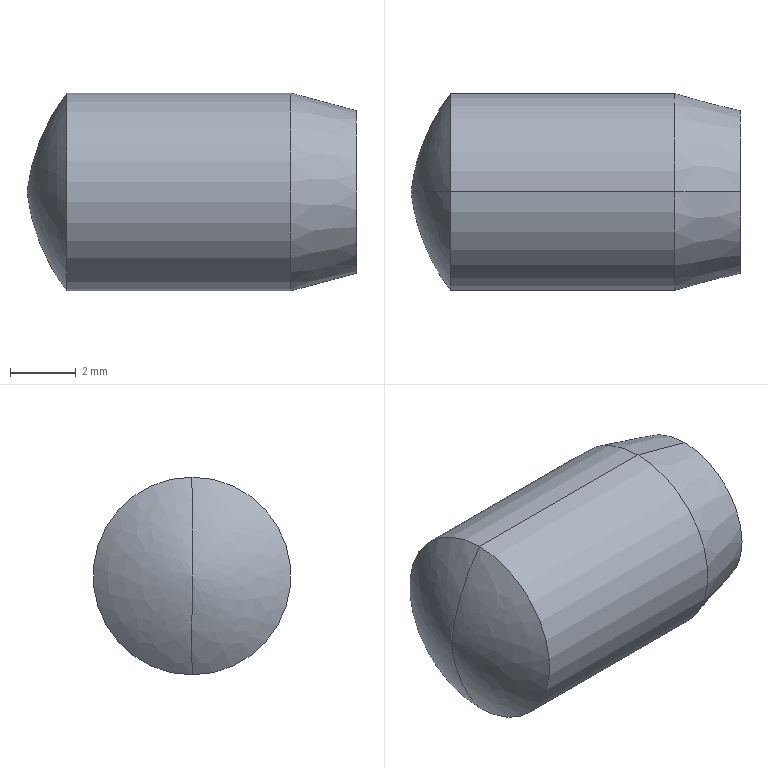Part | STEP file | 0245_020_MSC6-10 | 1 solid | 7 faces | box 10 x 6 x 6 mm | volume 255.239 mm3 | spline 2 | cylinder 2 | cone 2 | plane 1 | commonest cylinder face diameters 6 x2
STEP:
#1=CARTESIAN_POINT('',(0.,0.,0.));
#2=DIRECTION('',(0.,0.,1.));
#3=DIRECTION('',(1.,0.,0.));
#4=AXIS2_PLACEMENT_3D('',#1,#2,#3);
#5=CARTESIAN_POINT('',(-5.,0.,0.));
#6=VERTEX_POINT('',#5);
#7=CARTESIAN_POINT('',(-3.8,0.,3.));
#8=VERTEX_POINT('',#7);
#9=CARTESIAN_POINT('',(0.9651,0.,-0.646));
#10=DIRECTION('',(0.,1.,0.));
#11=DIRECTION('',(0.,0.,1.));
#12=AXIS2_PLACEMENT_3D('',#9,#10,#11);
#13=CIRCLE('',#12,6.);
#14=CARTESIAN_POINT('',(-5.,0.,0.));
#15=CARTESIAN_POINT('',(-5.,0.,0.));
#16=CARTESIAN_POINT('',(-5.,0.,0.));
#17=CARTESIAN_POINT('',(-5.,0.,0.));
#18=CARTESIAN_POINT('',(-4.881,0.,-1.098));
#19=CARTESIAN_POINT('',(-4.881,-2.196,-1.098));
#20=CARTESIAN_POINT('',(-4.881,-2.196,1.098));
#21=CARTESIAN_POINT('',(-4.881,0.,1.098));
#22=CARTESIAN_POINT('',(-4.471,0.,-2.123));
#23=CARTESIAN_POINT('',(-4.471,-4.246,-2.123));
#24=CARTESIAN_POINT('',(-4.471,-4.246,2.123));
#25=CARTESIAN_POINT('',(-4.471,0.,2.123));
#26=CARTESIAN_POINT('',(-3.8,0.,-3.));
#27=CARTESIAN_POINT('',(-3.8,-6.,-3.));
#28=CARTESIAN_POINT('',(-3.8,-6.,3.));
#29=CARTESIAN_POINT('',(-3.8,0.,3.));
#30=(BOUNDED_SURFACE()B_SPLINE_SURFACE(3,3,((#14,#15,#16,#17),(#18,#19,#20,#21),(#22,#23,#24,#25),(#26,#27,#28,#29)),.UNSPECIFIED.,.F.,.F.,.F.)B_SPLINE_SURFACE_WITH_KNOTS((4,4),(4,4),(0.,1.),(0.,1.),.PIECEWISE_BEZIER_KNOTS.)GEOMETRIC_REPRESENTATION_ITEM()RATIONAL_B_SPLINE_SURFACE(((1.,0.3333,0.3333,1.),(0.9754,0.3251,0.3251,0.9754),(0.9754,0.3251,0.3251,0.9754),(1.,0.3333,0.3333,1.)))REPRESENTATION_ITEM('')SURFACE());
#31=CARTESIAN_POINT('',(0.,1.));
#32=CARTESIAN_POINT('',(0.01534,1.));
#33=CARTESIAN_POINT('',(0.04597,1.));
#34=CARTESIAN_POINT('',(0.09177,1.));
#35=CARTESIAN_POINT('',(0.1374,1.));
#36=CARTESIAN_POINT('',(0.183,1.));
#37=CARTESIAN_POINT('',(0.2285,1.));
#38=CARTESIAN_POINT('',(0.2739,1.));
#39=CARTESIAN_POINT('',(0.3192,1.));
#40=CARTESIAN_POINT('',(0.3644,1.));
#41=CARTESIAN_POINT('',(0.4096,1.));
#42=CARTESIAN_POINT('',(0.4548,1.));
#43=CARTESIAN_POINT('',(0.5,1.));
#44=CARTESIAN_POINT('',(0.5452,1.));
#45=CARTESIAN_POINT('',(0.5904,1.));
#46=CARTESIAN_POINT('',(0.6356,1.));
#47=CARTESIAN_POINT('',(0.6808,1.));
#48=CARTESIAN_POINT('',(0.7261,1.));
#49=CARTESIAN_POINT('',(0.7715,1.));
#50=CARTESIAN_POINT('',(0.817,1.));
#51=CARTESIAN_POINT('',(0.8626,1.));
#52=CARTESIAN_POINT('',(0.9082,1.));
#53=CARTESIAN_POINT('',(0.954,1.));
#54=CARTESIAN_POINT('',(0.9847,1.));
#55=CARTESIAN_POINT('',(1.,1.));
#56=B_SPLINE_CURVE_WITH_KNOTS('',3,(#31,#32,#33,#34,#35,#36,#37,#38,#39,#40,#41,#42,#43,#44,#45,#46,#47,#48,#49,#50,#51,#52,#53,#54,#55),.UNSPECIFIED.,.F.,.F.,(4,1,1,1,1,1,1,1,1,1,1,1,1,1,1,1,1,1,1,1,1,1,4),(4.82,4.845,4.87,4.895,4.919,4.944,4.969,4.994,5.019,5.043,5.068,5.093,5.118,5.142,5.167,5.192,5.217,5.242,5.266,5.291,5.316,5.341,5.366),.QUASI_UNIFORM_KNOTS.);
#57=(GEOMETRIC_REPRESENTATION_CONTEXT(2)PARAMETRIC_REPRESENTATION_CONTEXT()REPRESENTATION_CONTEXT('',''));
#58=DEFINITIONAL_REPRESENTATION('',(#56),#57);
#59=PCURVE('',#30,#58);
#60=CARTESIAN_POINT('',(-5.,0.,0.));
#61=CARTESIAN_POINT('',(-5.,0.,0.));
#62=CARTESIAN_POINT('',(-5.,0.,0.));
#63=CARTESIAN_POINT('',(-5.,0.,0.));
#64=CARTESIAN_POINT('',(-4.881,0.,1.098));
#65=CARTESIAN_POINT('',(-4.881,2.196,1.098));
#66=CARTESIAN_POINT('',(-4.881,2.196,-1.098));
#67=CARTESIAN_POINT('',(-4.881,0.,-1.098));
#68=CARTESIAN_POINT('',(-4.471,0.,2.123));
#69=CARTESIAN_POINT('',(-4.471,4.246,2.123));
#70=CARTESIAN_POINT('',(-4.471,4.246,-2.123));
#71=CARTESIAN_POINT('',(-4.471,0.,-2.123));
#72=CARTESIAN_POINT('',(-3.8,0.,3.));
#73=CARTESIAN_POINT('',(-3.8,6.,3.));
#74=CARTESIAN_POINT('',(-3.8,6.,-3.));
#75=CARTESIAN_POINT('',(-3.8,0.,-3.));
#76=(BOUNDED_SURFACE()B_SPLINE_SURFACE(3,3,((#60,#61,#62,#63),(#64,#65,#66,#67),(#68,#69,#70,#71),(#72,#73,#74,#75)),.UNSPECIFIED.,.F.,.F.,.F.)B_SPLINE_SURFACE_WITH_KNOTS((4,4),(4,4),(0.,1.),(0.,1.),.PIECEWISE_BEZIER_KNOTS.)GEOMETRIC_REPRESENTATION_ITEM()RATIONAL_B_SPLINE_SURFACE(((1.,0.3333,0.3333,1.),(0.9754,0.3251,0.3251,0.9754),(0.9754,0.3251,0.3251,0.9754),(1.,0.3333,0.3333,1.)))REPRESENTATION_ITEM('')SURFACE());
#77=CARTESIAN_POINT('',(0.,0.));
#78=CARTESIAN_POINT('',(0.01534,0.));
#79=CARTESIAN_POINT('',(0.04597,0.));
#80=CARTESIAN_POINT('',(0.09177,0.));
#81=CARTESIAN_POINT('',(0.1374,0.));
#82=CARTESIAN_POINT('',(0.183,0.));
#83=CARTESIAN_POINT('',(0.2285,0.));
#84=CARTESIAN_POINT('',(0.2739,0.));
#85=CARTESIAN_POINT('',(0.3192,0.));
#86=CARTESIAN_POINT('',(0.3644,0.));
#87=CARTESIAN_POINT('',(0.4096,0.));
#88=CARTESIAN_POINT('',(0.4548,0.));
#89=CARTESIAN_POINT('',(0.5,0.));
#90=CARTESIAN_POINT('',(0.5452,0.));
#91=CARTESIAN_POINT('',(0.5904,0.));
#92=CARTESIAN_POINT('',(0.6356,0.));
#93=CARTESIAN_POINT('',(0.6808,0.));
#94=CARTESIAN_POINT('',(0.7261,0.));
#95=CARTESIAN_POINT('',(0.7715,0.));
#96=CARTESIAN_POINT('',(0.817,0.));
#97=CARTESIAN_POINT('',(0.8626,0.));
#98=CARTESIAN_POINT('',(0.9082,0.));
#99=CARTESIAN_POINT('',(0.954,0.));
#100=CARTESIAN_POINT('',(0.9847,0.));
#101=CARTESIAN_POINT('',(1.,0.));
#102=B_SPLINE_CURVE_WITH_KNOTS('',3,(#77,#78,#79,#80,#81,#82,#83,#84,#85,#86,#87,#88,#89,#90,#91,#92,#93,#94,#95,#96,#97,#98,#99,#100,#101),.UNSPECIFIED.,.F.,.F.,(4,1,1,1,1,1,1,1,1,1,1,1,1,1,1,1,1,1,1,1,1,1,4),(4.82,4.845,4.87,4.895,4.919,4.944,4.969,4.994,5.019,5.043,5.068,5.093,5.118,5.142,5.167,5.192,5.217,5.242,5.266,5.291,5.316,5.341,5.366),.QUASI_UNIFORM_KNOTS.);
#103=(GEOMETRIC_REPRESENTATION_CONTEXT(2)PARAMETRIC_REPRESENTATION_CONTEXT()REPRESENTATION_CONTEXT('',''));
#104=DEFINITIONAL_REPRESENTATION('',(#102),#103);
#105=PCURVE('',#76,#104);
#106=SURFACE_CURVE('',#13,(#59,#105),.PCURVE_S1.);
#107=EDGE_CURVE('',#6,#8,#106,.T.);
#108=ORIENTED_EDGE('',*,*,#107,.F.);
#109=CARTESIAN_POINT('',(-3.8,0.,-3.));
#110=VERTEX_POINT('',#109);
#111=CARTESIAN_POINT('',(0.9651,0.,0.646));
#112=DIRECTION('',(0.,-1.,0.));
#113=DIRECTION('',(0.,0.,-1.));
#114=AXIS2_PLACEMENT_3D('',#111,#112,#113);
#115=CIRCLE('',#114,6.);
#116=CARTESIAN_POINT('',(0.,0.));
#117=CARTESIAN_POINT('',(0.01534,0.));
#118=CARTESIAN_POINT('',(0.04597,0.));
#119=CARTESIAN_POINT('',(0.09177,0.));
#120=CARTESIAN_POINT('',(0.1374,0.));
#121=CARTESIAN_POINT('',(0.183,0.));
#122=CARTESIAN_POINT('',(0.2285,0.));
#123=CARTESIAN_POINT('',(0.2739,0.));
#124=CARTESIAN_POINT('',(0.3192,0.));
#125=CARTESIAN_POINT('',(0.3644,0.));
#126=CARTESIAN_POINT('',(0.4096,0.));
#127=CARTESIAN_POINT('',(0.4548,0.));
#128=CARTESIAN_POINT('',(0.5,0.));
#129=CARTESIAN_POINT('',(0.5452,0.));
#130=CARTESIAN_POINT('',(0.5904,0.));
#131=CARTESIAN_POINT('',(0.6356,0.));
#132=CARTESIAN_POINT('',(0.6808,0.));
#133=CARTESIAN_POINT('',(0.7261,0.));
#134=CARTESIAN_POINT('',(0.7715,0.));
#135=CARTESIAN_POINT('',(0.817,0.));
#136=CARTESIAN_POINT('',(0.8626,0.));
#137=CARTESIAN_POINT('',(0.9082,0.));
#138=CARTESIAN_POINT('',(0.954,0.));
#139=CARTESIAN_POINT('',(0.9847,0.));
#140=CARTESIAN_POINT('',(1.,0.));
#141=B_SPLINE_CURVE_WITH_KNOTS('',3,(#116,#117,#118,#119,#120,#121,#122,#123,#124,#125,#126,#127,#128,#129,#130,#131,#132,#133,#134,#135,#136,#137,#138,#139,#140),.UNSPECIFIED.,.F.,.F.,(4,1,1,1,1,1,1,1,1,1,1,1,1,1,1,1,1,1,1,1,1,1,4),(4.82,4.845,4.87,4.895,4.919,4.944,4.969,4.994,5.019,5.043,5.068,5.093,5.118,5.142,5.167,5.192,5.217,5.242,5.266,5.291,5.316,5.341,5.366),.QUASI_UNIFORM_KNOTS.);
#142=(GEOMETRIC_REPRESENTATION_CONTEXT(2)PARAMETRIC_REPRESENTATION_CONTEXT()REPRESENTATION_CONTEXT('',''));
#143=DEFINITIONAL_REPRESENTATION('',(#141),#142);
#144=PCURVE('',#30,#143);
#145=CARTESIAN_POINT('',(0.,1.));
#146=CARTESIAN_POINT('',(0.01534,1.));
#147=CARTESIAN_POINT('',(0.04597,1.));
#148=CARTESIAN_POINT('',(0.09177,1.));
#149=CARTESIAN_POINT('',(0.1374,1.));
#150=CARTESIAN_POINT('',(0.183,1.));
#151=CARTESIAN_POINT('',(0.2285,1.));
#152=CARTESIAN_POINT('',(0.2739,1.));
#153=CARTESIAN_POINT('',(0.3192,1.));
#154=CARTESIAN_POINT('',(0.3644,1.));
#155=CARTESIAN_POINT('',(0.4096,1.));
#156=CARTESIAN_POINT('',(0.4548,1.));
#157=CARTESIAN_POINT('',(0.5,1.));
#158=CARTESIAN_POINT('',(0.5452,1.));
#159=CARTESIAN_POINT('',(0.5904,1.));
#160=CARTESIAN_POINT('',(0.6356,1.));
#161=CARTESIAN_POINT('',(0.6808,1.));
#162=CARTESIAN_POINT('',(0.7261,1.));
#163=CARTESIAN_POINT('',(0.7715,1.));
#164=CARTESIAN_POINT('',(0.817,1.));
#165=CARTESIAN_POINT('',(0.8626,1.));
#166=CARTESIAN_POINT('',(0.9082,1.));
#167=CARTESIAN_POINT('',(0.954,1.));
#168=CARTESIAN_POINT('',(0.9847,1.));
#169=CARTESIAN_POINT('',(1.,1.));
#170=B_SPLINE_CURVE_WITH_KNOTS('',3,(#145,#146,#147,#148,#149,#150,#151,#152,#153,#154,#155,#156,#157,#158,#159,#160,#161,#162,#163,#164,#165,#166,#167,#168,#169),.UNSPECIFIED.,.F.,.F.,(4,1,1,1,1,1,1,1,1,1,1,1,1,1,1,1,1,1,1,1,1,1,4),(4.82,4.845,4.87,4.895,4.919,4.944,4.969,4.994,5.019,5.043,5.068,5.093,5.118,5.142,5.167,5.192,5.217,5.242,5.266,5.291,5.316,5.341,5.366),.QUASI_UNIFORM_KNOTS.);
#171=(GEOMETRIC_REPRESENTATION_CONTEXT(2)PARAMETRIC_REPRESENTATION_CONTEXT()REPRESENTATION_CONTEXT('',''));
#172=DEFINITIONAL_REPRESENTATION('',(#170),#171);
#173=PCURVE('',#76,#172);
#174=SURFACE_CURVE('',#115,(#144,#173),.PCURVE_S1.);
#175=EDGE_CURVE('',#6,#110,#174,.T.);
#176=ORIENTED_EDGE('',*,*,#175,.T.);
#177=CARTESIAN_POINT('',(-3.8,0.,0.));
#178=DIRECTION('',(1.,0.,0.));
#179=DIRECTION('',(0.,0.,-1.));
#180=AXIS2_PLACEMENT_3D('',#177,#178,#179);
#181=CIRCLE('',#180,3.);
#182=CARTESIAN_POINT('',(1.,1.));
#183=CARTESIAN_POINT('',(1.,0.9763));
#184=CARTESIAN_POINT('',(1.,0.9319));
#185=CARTESIAN_POINT('',(1.,0.8733));
#186=CARTESIAN_POINT('',(1.,0.8206));
#187=CARTESIAN_POINT('',(1.,0.7724));
#188=CARTESIAN_POINT('',(1.,0.7279));
#189=CARTESIAN_POINT('',(1.,0.6861));
#190=CARTESIAN_POINT('',(1.,0.6465));
#191=CARTESIAN_POINT('',(1.,0.6086));
#192=CARTESIAN_POINT('',(1.,0.5718));
#193=CARTESIAN_POINT('',(1.,0.5357));
#194=CARTESIAN_POINT('',(1.,0.5));
#195=CARTESIAN_POINT('',(1.,0.4643));
#196=CARTESIAN_POINT('',(1.,0.4282));
#197=CARTESIAN_POINT('',(1.,0.3914));
#198=CARTESIAN_POINT('',(1.,0.3535));
#199=CARTESIAN_POINT('',(1.,0.3139));
#200=CARTESIAN_POINT('',(1.,0.2721));
#201=CARTESIAN_POINT('',(1.,0.2276));
#202=CARTESIAN_POINT('',(1.,0.1794));
#203=CARTESIAN_POINT('',(1.,0.1267));
#204=CARTESIAN_POINT('',(1.,0.06805));
#205=CARTESIAN_POINT('',(1.,0.02375));
#206=CARTESIAN_POINT('',(1.,0.));
#207=B_SPLINE_CURVE_WITH_KNOTS('',3,(#182,#183,#184,#185,#186,#187,#188,#189,#190,#191,#192,#193,#194,#195,#196,#197,#198,#199,#200,#201,#202,#203,#204,#205,#206),.UNSPECIFIED.,.F.,.F.,(4,1,1,1,1,1,1,1,1,1,1,1,1,1,1,1,1,1,1,1,1,1,4),(3.142,3.284,3.427,3.57,3.713,3.856,3.998,4.141,4.284,4.427,4.57,4.712,4.855,4.998,5.141,5.284,5.426,5.569,5.712,5.855,5.998,6.14,6.283),.QUASI_UNIFORM_KNOTS.);
#208=(GEOMETRIC_REPRESENTATION_CONTEXT(2)PARAMETRIC_REPRESENTATION_CONTEXT()REPRESENTATION_CONTEXT('',''));
#209=DEFINITIONAL_REPRESENTATION('',(#207),#208);
#210=PCURVE('',#30,#209);
#211=CARTESIAN_POINT('',(-0.4,0.,0.));
#212=DIRECTION('',(1.,0.,0.));
#213=DIRECTION('',(0.,0.,-1.));
#214=AXIS2_PLACEMENT_3D('',#211,#212,#213);
#215=CYLINDRICAL_SURFACE('',#214,3.);
#216=CARTESIAN_POINT('',(0.,-3.4));
#217=DIRECTION('',(1.,0.));
#218=VECTOR('',#217,1.);
#219=LINE('',#216,#218);
#220=(GEOMETRIC_REPRESENTATION_CONTEXT(2)PARAMETRIC_REPRESENTATION_CONTEXT()REPRESENTATION_CONTEXT('',''));
#221=DEFINITIONAL_REPRESENTATION('',(#219),#220);
#222=PCURVE('',#215,#221);
#223=SURFACE_CURVE('',#181,(#210,#222),.PCURVE_S1.);
#224=EDGE_CURVE('',#8,#110,#223,.T.);
#225=ORIENTED_EDGE('',*,*,#224,.F.);
#226=EDGE_LOOP('',(#108,#176,#225));
#227=FACE_BOUND('',#226,.T.);
#228=ADVANCED_FACE('',(#227),#30,.T.);
#229=CARTESIAN_POINT('',(-3.8,0.,0.));
#230=DIRECTION('',(1.,0.,0.));
#231=DIRECTION('',(0.,0.,-1.));
#232=AXIS2_PLACEMENT_3D('',#229,#230,#231);
#233=CIRCLE('',#232,3.);
#234=CARTESIAN_POINT('',(-0.4,0.,0.));
#235=DIRECTION('',(1.,0.,0.));
#236=DIRECTION('',(0.,0.,-1.));
#237=AXIS2_PLACEMENT_3D('',#234,#235,#236);
#238=CYLINDRICAL_SURFACE('',#237,3.);
#239=CARTESIAN_POINT('',(0.,-3.4));
#240=DIRECTION('',(1.,0.));
#241=VECTOR('',#240,1.);
#242=LINE('',#239,#241);
#243=(GEOMETRIC_REPRESENTATION_CONTEXT(2)PARAMETRIC_REPRESENTATION_CONTEXT()REPRESENTATION_CONTEXT('',''));
#244=DEFINITIONAL_REPRESENTATION('',(#242),#243);
#245=PCURVE('',#238,#244);
#246=CARTESIAN_POINT('',(1.,1.));
#247=CARTESIAN_POINT('',(1.,0.9763));
#248=CARTESIAN_POINT('',(1.,0.9319));
#249=CARTESIAN_POINT('',(1.,0.8733));
#250=CARTESIAN_POINT('',(1.,0.8206));
#251=CARTESIAN_POINT('',(1.,0.7724));
#252=CARTESIAN_POINT('',(1.,0.7279));
#253=CARTESIAN_POINT('',(1.,0.6861));
#254=CARTESIAN_POINT('',(1.,0.6465));
#255=CARTESIAN_POINT('',(1.,0.6086));
#256=CARTESIAN_POINT('',(1.,0.5718));
#257=CARTESIAN_POINT('',(1.,0.5357));
#258=CARTESIAN_POINT('',(1.,0.5));
#259=CARTESIAN_POINT('',(1.,0.4643));
#260=CARTESIAN_POINT('',(1.,0.4282));
#261=CARTESIAN_POINT('',(1.,0.3914));
#262=CARTESIAN_POINT('',(1.,0.3535));
#263=CARTESIAN_POINT('',(1.,0.3139));
#264=CARTESIAN_POINT('',(1.,0.2721));
#265=CARTESIAN_POINT('',(1.,0.2276));
#266=CARTESIAN_POINT('',(1.,0.1794));
#267=CARTESIAN_POINT('',(1.,0.1267));
#268=CARTESIAN_POINT('',(1.,0.06805));
#269=CARTESIAN_POINT('',(1.,0.02375));
#270=CARTESIAN_POINT('',(1.,0.));
#271=B_SPLINE_CURVE_WITH_KNOTS('',3,(#246,#247,#248,#249,#250,#251,#252,#253,#254,#255,#256,#257,#258,#259,#260,#261,#262,#263,#264,#265,#266,#267,#268,#269,#270),.UNSPECIFIED.,.F.,.F.,(4,1,1,1,1,1,1,1,1,1,1,1,1,1,1,1,1,1,1,1,1,1,4),(0.,0.1428,0.2856,0.4284,0.5712,0.714,0.8568,0.9996,1.142,1.285,1.428,1.571,1.714,1.856,1.999,2.142,2.285,2.428,2.57,2.713,2.856,2.999,3.142),.QUASI_UNIFORM_KNOTS.);
#272=(GEOMETRIC_REPRESENTATION_CONTEXT(2)PARAMETRIC_REPRESENTATION_CONTEXT()REPRESENTATION_CONTEXT('',''));
#273=DEFINITIONAL_REPRESENTATION('',(#271),#272);
#274=PCURVE('',#76,#273);
#275=SURFACE_CURVE('',#233,(#245,#274),.PCURVE_S1.);
#276=EDGE_CURVE('',#110,#8,#275,.T.);
#277=ORIENTED_EDGE('',*,*,#276,.T.);
#278=CARTESIAN_POINT('',(3.,0.,3.));
#279=VERTEX_POINT('',#278);
#280=CARTESIAN_POINT('',(-0.4,0.,3.));
#281=DIRECTION('',(1.,0.,0.));
#282=VECTOR('',#281,1.);
#283=LINE('',#280,#282);
#284=CARTESIAN_POINT('',(3.142,0.));
#285=DIRECTION('',(0.,1.));
#286=VECTOR('',#285,1.);
#287=LINE('',#284,#286);
#288=(GEOMETRIC_REPRESENTATION_CONTEXT(2)PARAMETRIC_REPRESENTATION_CONTEXT()REPRESENTATION_CONTEXT('',''));
#289=DEFINITIONAL_REPRESENTATION('',(#287),#288);
#290=PCURVE('',#238,#289);
#291=CARTESIAN_POINT('',(3.142,0.));
#292=DIRECTION('',(0.,1.));
#293=VECTOR('',#292,1.);
#294=LINE('',#291,#293);
#295=(GEOMETRIC_REPRESENTATION_CONTEXT(2)PARAMETRIC_REPRESENTATION_CONTEXT()REPRESENTATION_CONTEXT('',''));
#296=DEFINITIONAL_REPRESENTATION('',(#294),#295);
#297=PCURVE('',#215,#296);
#298=SURFACE_CURVE('',#283,(#290,#297),.PCURVE_S1.);
#299=EDGE_CURVE('',#8,#279,#298,.T.);
#300=ORIENTED_EDGE('',*,*,#299,.T.);
#301=CARTESIAN_POINT('',(3.,0.,-3.));
#302=VERTEX_POINT('',#301);
#303=CARTESIAN_POINT('',(3.,0.,0.));
#304=DIRECTION('',(-1.,0.,0.));
#305=DIRECTION('',(0.,0.,-1.));
#306=AXIS2_PLACEMENT_3D('',#303,#304,#305);
#307=CIRCLE('',#306,3.);
#308=CARTESIAN_POINT('',(6.283,3.4));
#309=DIRECTION('',(-1.,0.));
#310=VECTOR('',#309,1.);
#311=LINE('',#308,#310);
#312=(GEOMETRIC_REPRESENTATION_CONTEXT(2)PARAMETRIC_REPRESENTATION_CONTEXT()REPRESENTATION_CONTEXT('',''));
#313=DEFINITIONAL_REPRESENTATION('',(#311),#312);
#314=PCURVE('',#238,#313);
#315=CARTESIAN_POINT('',(3.,0.,0.));
#316=DIRECTION('',(-1.,0.,0.));
#317=DIRECTION('',(0.,0.,1.));
#318=AXIS2_PLACEMENT_3D('',#315,#316,#317);
#319=CONICAL_SURFACE('',#318,3.,0.2618);
#320=CARTESIAN_POINT('',(-3.142,0.));
#321=DIRECTION('',(1.,0.));
#322=VECTOR('',#321,1.);
#323=LINE('',#320,#322);
#324=(GEOMETRIC_REPRESENTATION_CONTEXT(2)PARAMETRIC_REPRESENTATION_CONTEXT()REPRESENTATION_CONTEXT('',''));
#325=DEFINITIONAL_REPRESENTATION('',(#323),#324);
#326=PCURVE('',#319,#325);
#327=SURFACE_CURVE('',#307,(#314,#326),.PCURVE_S1.);
#328=EDGE_CURVE('',#279,#302,#327,.T.);
#329=ORIENTED_EDGE('',*,*,#328,.T.);
#330=CARTESIAN_POINT('',(-0.4,0.,-3.));
#331=DIRECTION('',(1.,0.,0.));
#332=VECTOR('',#331,1.);
#333=LINE('',#330,#332);
#334=CARTESIAN_POINT('',(0.,0.));
#335=DIRECTION('',(0.,1.));
#336=VECTOR('',#335,1.);
#337=LINE('',#334,#336);
#338=(GEOMETRIC_REPRESENTATION_CONTEXT(2)PARAMETRIC_REPRESENTATION_CONTEXT()REPRESENTATION_CONTEXT('',''));
#339=DEFINITIONAL_REPRESENTATION('',(#337),#338);
#340=PCURVE('',#238,#339);
#341=CARTESIAN_POINT('',(6.283,0.));
#342=DIRECTION('',(0.,1.));
#343=VECTOR('',#342,1.);
#344=LINE('',#341,#343);
#345=(GEOMETRIC_REPRESENTATION_CONTEXT(2)PARAMETRIC_REPRESENTATION_CONTEXT()REPRESENTATION_CONTEXT('',''));
#346=DEFINITIONAL_REPRESENTATION('',(#344),#345);
#347=PCURVE('',#215,#346);
#348=SURFACE_CURVE('',#333,(#340,#347),.PCURVE_S1.);
#349=EDGE_CURVE('',#110,#302,#348,.T.);
#350=ORIENTED_EDGE('',*,*,#349,.F.);
#351=EDGE_LOOP('',(#277,#300,#329,#350));
#352=FACE_BOUND('',#351,.T.);
#353=ADVANCED_FACE('',(#352),#238,.T.);
#354=CARTESIAN_POINT('',(5.,0.,2.464));
#355=VERTEX_POINT('',#354);
#356=CARTESIAN_POINT('',(5.,0.,-2.464));
#357=VERTEX_POINT('',#356);
#358=CARTESIAN_POINT('',(5.,0.,0.));
#359=DIRECTION('',(-1.,0.,0.));
#360=DIRECTION('',(0.,0.,1.));
#361=AXIS2_PLACEMENT_3D('',#358,#359,#360);
#362=CIRCLE('',#361,2.464);
#363=CARTESIAN_POINT('',(0.,-2.));
#364=DIRECTION('',(1.,0.));
#365=VECTOR('',#364,1.);
#366=LINE('',#363,#365);
#367=(GEOMETRIC_REPRESENTATION_CONTEXT(2)PARAMETRIC_REPRESENTATION_CONTEXT()REPRESENTATION_CONTEXT('',''));
#368=DEFINITIONAL_REPRESENTATION('',(#366),#367);
#369=PCURVE('',#319,#368);
#370=CARTESIAN_POINT('',(5.,1.232,0.));
#371=DIRECTION('',(1.,0.,0.));
#372=DIRECTION('',(0.,0.,-1.));
#373=AXIS2_PLACEMENT_3D('',#370,#371,#372);
#374=PLANE('',#373);
#375=CARTESIAN_POINT('',(-2.464,-1.232));
#376=CARTESIAN_POINT('',(-2.464,3.036));
#377=CARTESIAN_POINT('',(1.232,0.9019));
#378=CARTESIAN_POINT('',(4.928,-1.232));
#379=CARTESIAN_POINT('',(1.232,-3.366));
#380=CARTESIAN_POINT('',(-2.464,-5.5));
#381=CARTESIAN_POINT('',(-2.464,-1.232));
#382=(BOUNDED_CURVE()B_SPLINE_CURVE(2,(#375,#376,#377,#378,#379,#380,#381),.UNSPECIFIED.,.T.,.F.)B_SPLINE_CURVE_WITH_KNOTS((1,2,2,2,2,1),(-2.094,0.,2.094,4.189,6.283,8.378),.UNSPECIFIED.)CURVE()GEOMETRIC_REPRESENTATION_ITEM()RATIONAL_B_SPLINE_CURVE((1.,0.5,1.,0.5,1.,0.5,1.))REPRESENTATION_ITEM(''));
#383=(GEOMETRIC_REPRESENTATION_CONTEXT(2)PARAMETRIC_REPRESENTATION_CONTEXT()REPRESENTATION_CONTEXT('',''));
#384=DEFINITIONAL_REPRESENTATION('',(#382),#383);
#385=PCURVE('',#374,#384);
#386=SURFACE_CURVE('',#362,(#369,#385),.PCURVE_S1.);
#387=EDGE_CURVE('',#355,#357,#386,.T.);
#388=ORIENTED_EDGE('',*,*,#387,.T.);
#389=CARTESIAN_POINT('',(3.,0.,-3.));
#390=DIRECTION('',(-0.9659,0.,-0.2588));
#391=VECTOR('',#390,1.);
#392=LINE('',#389,#391);
#393=CARTESIAN_POINT('',(3.142,0.));
#394=DIRECTION('',(0.,1.));
#395=VECTOR('',#394,1.);
#396=LINE('',#393,#395);
#397=(GEOMETRIC_REPRESENTATION_CONTEXT(2)PARAMETRIC_REPRESENTATION_CONTEXT()REPRESENTATION_CONTEXT('',''));
#398=DEFINITIONAL_REPRESENTATION('',(#396),#397);
#399=PCURVE('',#319,#398);
#400=CARTESIAN_POINT('',(3.,0.,0.));
#401=DIRECTION('',(-1.,0.,0.));
#402=DIRECTION('',(0.,0.,1.));
#403=AXIS2_PLACEMENT_3D('',#400,#401,#402);
#404=CONICAL_SURFACE('',#403,3.,0.2618);
#405=CARTESIAN_POINT('',(3.142,0.));
#406=DIRECTION('',(0.,1.));
#407=VECTOR('',#406,1.);
#408=LINE('',#405,#407);
#409=(GEOMETRIC_REPRESENTATION_CONTEXT(2)PARAMETRIC_REPRESENTATION_CONTEXT()REPRESENTATION_CONTEXT('',''));
#410=DEFINITIONAL_REPRESENTATION('',(#408),#409);
#411=PCURVE('',#404,#410);
#412=SURFACE_CURVE('',#392,(#399,#411),.PCURVE_S1.);
#413=EDGE_CURVE('',#357,#302,#412,.T.);
#414=ORIENTED_EDGE('',*,*,#413,.T.);
#415=ORIENTED_EDGE('',*,*,#328,.F.);
#416=CARTESIAN_POINT('',(3.,0.,3.));
#417=DIRECTION('',(-0.9659,0.,0.2588));
#418=VECTOR('',#417,1.);
#419=LINE('',#416,#418);
#420=CARTESIAN_POINT('',(0.,0.));
#421=DIRECTION('',(0.,1.));
#422=VECTOR('',#421,1.);
#423=LINE('',#420,#422);
#424=(GEOMETRIC_REPRESENTATION_CONTEXT(2)PARAMETRIC_REPRESENTATION_CONTEXT()REPRESENTATION_CONTEXT('',''));
#425=DEFINITIONAL_REPRESENTATION('',(#423),#424);
#426=PCURVE('',#319,#425);
#427=CARTESIAN_POINT('',(6.283,0.));
#428=DIRECTION('',(0.,1.));
#429=VECTOR('',#428,1.);
#430=LINE('',#427,#429);
#431=(GEOMETRIC_REPRESENTATION_CONTEXT(2)PARAMETRIC_REPRESENTATION_CONTEXT()REPRESENTATION_CONTEXT('',''));
#432=DEFINITIONAL_REPRESENTATION('',(#430),#431);
#433=PCURVE('',#404,#432);
#434=SURFACE_CURVE('',#419,(#426,#433),.PCURVE_S1.);
#435=EDGE_CURVE('',#355,#279,#434,.T.);
#436=ORIENTED_EDGE('',*,*,#435,.F.);
#437=EDGE_LOOP('',(#388,#414,#415,#436));
#438=FACE_BOUND('',#437,.T.);
#439=ADVANCED_FACE('',(#438),#319,.T.);
#440=ORIENTED_EDGE('',*,*,#299,.F.);
#441=ORIENTED_EDGE('',*,*,#224,.T.);
#442=ORIENTED_EDGE('',*,*,#349,.T.);
#443=CARTESIAN_POINT('',(3.,0.,0.));
#444=DIRECTION('',(-1.,0.,0.));
#445=DIRECTION('',(0.,0.,-1.));
#446=AXIS2_PLACEMENT_3D('',#443,#444,#445);
#447=CIRCLE('',#446,3.);
#448=CARTESIAN_POINT('',(6.283,3.4));
#449=DIRECTION('',(-1.,0.));
#450=VECTOR('',#449,1.);
#451=LINE('',#448,#450);
#452=(GEOMETRIC_REPRESENTATION_CONTEXT(2)PARAMETRIC_REPRESENTATION_CONTEXT()REPRESENTATION_CONTEXT('',''));
#453=DEFINITIONAL_REPRESENTATION('',(#451),#452);
#454=PCURVE('',#215,#453);
#455=CARTESIAN_POINT('',(3.142,0.));
#456=DIRECTION('',(1.,0.));
#457=VECTOR('',#456,1.);
#458=LINE('',#455,#457);
#459=(GEOMETRIC_REPRESENTATION_CONTEXT(2)PARAMETRIC_REPRESENTATION_CONTEXT()REPRESENTATION_CONTEXT('',''));
#460=DEFINITIONAL_REPRESENTATION('',(#458),#459);
#461=PCURVE('',#404,#460);
#462=SURFACE_CURVE('',#447,(#454,#461),.PCURVE_S1.);
#463=EDGE_CURVE('',#302,#279,#462,.T.);
#464=ORIENTED_EDGE('',*,*,#463,.T.);
#465=EDGE_LOOP('',(#440,#441,#442,#464));
#466=FACE_BOUND('',#465,.T.);
#467=ADVANCED_FACE('',(#466),#215,.T.);
#468=ORIENTED_EDGE('',*,*,#175,.F.);
#469=ORIENTED_EDGE('',*,*,#107,.T.);
#470=ORIENTED_EDGE('',*,*,#276,.F.);
#471=EDGE_LOOP('',(#468,#469,#470));
#472=FACE_BOUND('',#471,.T.);
#473=ADVANCED_FACE('',(#472),#76,.T.);
#474=ORIENTED_EDGE('',*,*,#413,.F.);
#475=CARTESIAN_POINT('',(5.,0.,0.));
#476=DIRECTION('',(-1.,0.,0.));
#477=DIRECTION('',(0.,0.,1.));
#478=AXIS2_PLACEMENT_3D('',#475,#476,#477);
#479=CIRCLE('',#478,2.464);
#480=CARTESIAN_POINT('',(0.,-2.));
#481=DIRECTION('',(1.,0.));
#482=VECTOR('',#481,1.);
#483=LINE('',#480,#482);
#484=(GEOMETRIC_REPRESENTATION_CONTEXT(2)PARAMETRIC_REPRESENTATION_CONTEXT()REPRESENTATION_CONTEXT('',''));
#485=DEFINITIONAL_REPRESENTATION('',(#483),#484);
#486=PCURVE('',#404,#485);
#487=CARTESIAN_POINT('',(-2.464,-1.232));
#488=CARTESIAN_POINT('',(-2.464,3.036));
#489=CARTESIAN_POINT('',(1.232,0.9019));
#490=CARTESIAN_POINT('',(4.928,-1.232));
#491=CARTESIAN_POINT('',(1.232,-3.366));
#492=CARTESIAN_POINT('',(-2.464,-5.5));
#493=CARTESIAN_POINT('',(-2.464,-1.232));
#494=(BOUNDED_CURVE()B_SPLINE_CURVE(2,(#487,#488,#489,#490,#491,#492,#493),.UNSPECIFIED.,.T.,.F.)B_SPLINE_CURVE_WITH_KNOTS((1,2,2,2,2,1),(-2.094,0.,2.094,4.189,6.283,8.378),.UNSPECIFIED.)CURVE()GEOMETRIC_REPRESENTATION_ITEM()RATIONAL_B_SPLINE_CURVE((1.,0.5,1.,0.5,1.,0.5,1.))REPRESENTATION_ITEM(''));
#495=(GEOMETRIC_REPRESENTATION_CONTEXT(2)PARAMETRIC_REPRESENTATION_CONTEXT()REPRESENTATION_CONTEXT('',''));
#496=DEFINITIONAL_REPRESENTATION('',(#494),#495);
#497=PCURVE('',#374,#496);
#498=SURFACE_CURVE('',#479,(#486,#497),.PCURVE_S1.);
#499=EDGE_CURVE('',#357,#355,#498,.T.);
#500=ORIENTED_EDGE('',*,*,#499,.T.);
#501=ORIENTED_EDGE('',*,*,#435,.T.);
#502=ORIENTED_EDGE('',*,*,#463,.F.);
#503=EDGE_LOOP('',(#474,#500,#501,#502));
#504=FACE_BOUND('',#503,.T.);
#505=ADVANCED_FACE('',(#504),#404,.T.);
#506=ORIENTED_EDGE('',*,*,#387,.F.);
#507=ORIENTED_EDGE('',*,*,#499,.F.);
#508=EDGE_LOOP('',(#506,#507));
#509=FACE_BOUND('',#508,.T.);
#510=ADVANCED_FACE('',(#509),#374,.T.);
#511=CLOSED_SHELL('',(#228,#353,#439,#467,#473,#505,#510));
#512=MANIFOLD_SOLID_BREP('',#511);
#513=(LENGTH_UNIT()NAMED_UNIT(*)SI_UNIT(.MILLI.,.METRE.));
#514=UNCERTAINTY_MEASURE_WITH_UNIT(LENGTH_MEASURE(0.0000001),#513,'','');
#515=(NAMED_UNIT(*)PLANE_ANGLE_UNIT()SI_UNIT($,.RADIAN.));
#516=(NAMED_UNIT(*)SI_UNIT($,.STERADIAN.)SOLID_ANGLE_UNIT());
#517=(GEOMETRIC_REPRESENTATION_CONTEXT(3)GLOBAL_UNCERTAINTY_ASSIGNED_CONTEXT((#514))GLOBAL_UNIT_ASSIGNED_CONTEXT((#513,#515,#516))REPRESENTATION_CONTEXT('',''));
#518=ADVANCED_BREP_SHAPE_REPRESENTATION('',(#4,#512),#517);